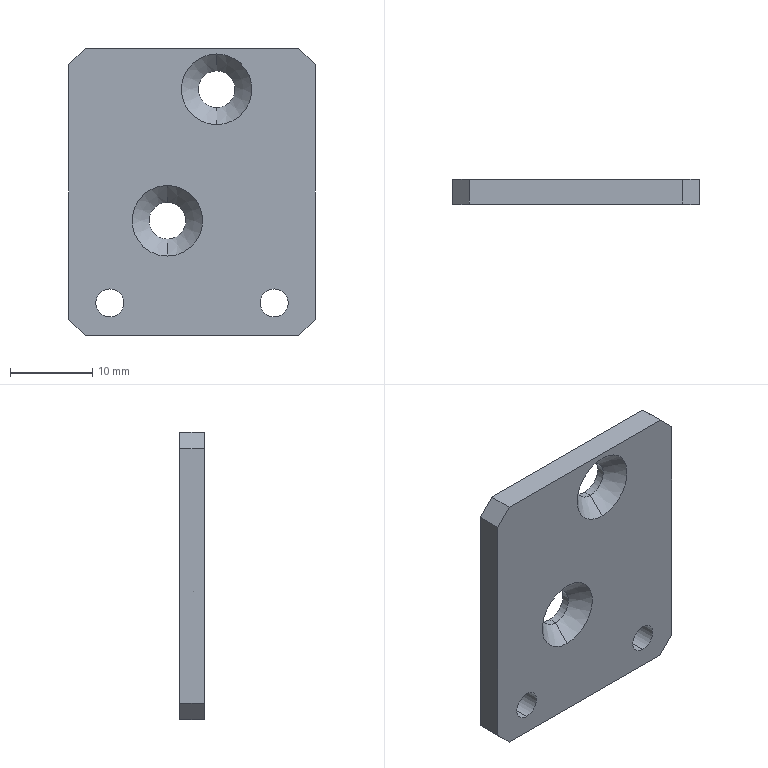Part | NX | features BREP 1 | 1 solid | 22 faces | box 30 x 3 x 35 mm | volume 2899 mm3 | plane 10 | cylinder 8 | cone 4 | commonest cylinder face diameters 3.4 x4 4.5 x4
STEP:
#1=CARTESIAN_POINT('',(-15.,-3.,-15.5));
#2=VERTEX_POINT('',#1);
#3=CARTESIAN_POINT('',(-13.,-3.,-17.5));
#4=VERTEX_POINT('',#3);
#5=CARTESIAN_POINT('',(-13.,-3.,-17.5));
#6=DIRECTION('',(0.7071,0.,-0.7071));
#7=VECTOR('',#6,1000.);
#8=LINE('',#5,#7);
#9=EDGE_CURVE('',#2,#4,#8,.T.);
#10=ORIENTED_EDGE('',*,*,#9,.F.);
#11=CARTESIAN_POINT('',(-15.,0.,-15.5));
#12=VERTEX_POINT('',#11);
#13=CARTESIAN_POINT('',(-15.,-3.,-15.5));
#14=DIRECTION('',(0.,-1.,0.));
#15=VECTOR('',#14,1000.);
#16=LINE('',#13,#15);
#17=EDGE_CURVE('',#12,#2,#16,.T.);
#18=ORIENTED_EDGE('',*,*,#17,.F.);
#19=CARTESIAN_POINT('',(-13.,0.,-17.5));
#20=VERTEX_POINT('',#19);
#21=CARTESIAN_POINT('',(-15.25,0.,-15.25));
#22=DIRECTION('',(-0.7071,0.,0.7071));
#23=VECTOR('',#22,1000.);
#24=LINE('',#21,#23);
#25=EDGE_CURVE('',#20,#12,#24,.T.);
#26=ORIENTED_EDGE('',*,*,#25,.F.);
#27=CARTESIAN_POINT('',(-13.,-3.,-17.5));
#28=DIRECTION('',(0.,1.,0.));
#29=VECTOR('',#28,1000.);
#30=LINE('',#27,#29);
#31=EDGE_CURVE('',#4,#20,#30,.T.);
#32=ORIENTED_EDGE('',*,*,#31,.F.);
#33=EDGE_LOOP('',(#10,#18,#26,#32));
#34=FACE_BOUND('',#33,.T.);
#35=CARTESIAN_POINT('',(-13.,-3.,-17.5));
#36=DIRECTION('',(0.7071,0.,0.7071));
#37=DIRECTION('',(0.,1.,0.));
#38=AXIS2_PLACEMENT_3D('',#35,#36,#37);
#39=PLANE('',#38);
#40=ADVANCED_FACE('',(#34),#39,.F.);
#41=CARTESIAN_POINT('',(13.,-3.,-17.5));
#42=VERTEX_POINT('',#41);
#43=CARTESIAN_POINT('',(15.,-3.,-15.5));
#44=VERTEX_POINT('',#43);
#45=CARTESIAN_POINT('',(15.,-3.,-15.5));
#46=DIRECTION('',(0.7071,0.,0.7071));
#47=VECTOR('',#46,1000.);
#48=LINE('',#45,#47);
#49=EDGE_CURVE('',#42,#44,#48,.T.);
#50=ORIENTED_EDGE('',*,*,#49,.F.);
#51=CARTESIAN_POINT('',(13.,0.,-17.5));
#52=VERTEX_POINT('',#51);
#53=CARTESIAN_POINT('',(13.,-3.,-17.5));
#54=DIRECTION('',(0.,-1.,0.));
#55=VECTOR('',#54,1000.);
#56=LINE('',#53,#55);
#57=EDGE_CURVE('',#52,#42,#56,.T.);
#58=ORIENTED_EDGE('',*,*,#57,.F.);
#59=CARTESIAN_POINT('',(15.,0.,-15.5));
#60=VERTEX_POINT('',#59);
#61=CARTESIAN_POINT('',(15.25,0.,-15.25));
#62=DIRECTION('',(-0.7071,0.,-0.7071));
#63=VECTOR('',#62,1000.);
#64=LINE('',#61,#63);
#65=EDGE_CURVE('',#60,#52,#64,.T.);
#66=ORIENTED_EDGE('',*,*,#65,.F.);
#67=CARTESIAN_POINT('',(15.,-3.,-15.5));
#68=DIRECTION('',(0.,1.,0.));
#69=VECTOR('',#68,1000.);
#70=LINE('',#67,#69);
#71=EDGE_CURVE('',#44,#60,#70,.T.);
#72=ORIENTED_EDGE('',*,*,#71,.F.);
#73=EDGE_LOOP('',(#50,#58,#66,#72));
#74=FACE_BOUND('',#73,.T.);
#75=CARTESIAN_POINT('',(15.,-3.,-15.5));
#76=DIRECTION('',(-0.7071,0.,0.7071));
#77=DIRECTION('',(0.,1.,0.));
#78=AXIS2_PLACEMENT_3D('',#75,#76,#77);
#79=PLANE('',#78);
#80=ADVANCED_FACE('',(#74),#79,.F.);
#81=CARTESIAN_POINT('',(15.,-3.,15.5));
#82=VERTEX_POINT('',#81);
#83=CARTESIAN_POINT('',(13.,-3.,17.5));
#84=VERTEX_POINT('',#83);
#85=CARTESIAN_POINT('',(13.,-3.,17.5));
#86=DIRECTION('',(-0.7071,0.,0.7071));
#87=VECTOR('',#86,1000.);
#88=LINE('',#85,#87);
#89=EDGE_CURVE('',#82,#84,#88,.T.);
#90=ORIENTED_EDGE('',*,*,#89,.F.);
#91=CARTESIAN_POINT('',(15.,0.,15.5));
#92=VERTEX_POINT('',#91);
#93=CARTESIAN_POINT('',(15.,-3.,15.5));
#94=DIRECTION('',(0.,-1.,0.));
#95=VECTOR('',#94,1000.);
#96=LINE('',#93,#95);
#97=EDGE_CURVE('',#92,#82,#96,.T.);
#98=ORIENTED_EDGE('',*,*,#97,.F.);
#99=CARTESIAN_POINT('',(13.,0.,17.5));
#100=VERTEX_POINT('',#99);
#101=CARTESIAN_POINT('',(15.25,0.,15.25));
#102=DIRECTION('',(0.7071,0.,-0.7071));
#103=VECTOR('',#102,1000.);
#104=LINE('',#101,#103);
#105=EDGE_CURVE('',#100,#92,#104,.T.);
#106=ORIENTED_EDGE('',*,*,#105,.F.);
#107=CARTESIAN_POINT('',(13.,-3.,17.5));
#108=DIRECTION('',(0.,1.,0.));
#109=VECTOR('',#108,1000.);
#110=LINE('',#107,#109);
#111=EDGE_CURVE('',#84,#100,#110,.T.);
#112=ORIENTED_EDGE('',*,*,#111,.F.);
#113=EDGE_LOOP('',(#90,#98,#106,#112));
#114=FACE_BOUND('',#113,.T.);
#115=CARTESIAN_POINT('',(13.,-3.,17.5));
#116=DIRECTION('',(-0.7071,0.,-0.7071));
#117=DIRECTION('',(0.,1.,0.));
#118=AXIS2_PLACEMENT_3D('',#115,#116,#117);
#119=PLANE('',#118);
#120=ADVANCED_FACE('',(#114),#119,.F.);
#121=CARTESIAN_POINT('',(-13.,-3.,17.5));
#122=VERTEX_POINT('',#121);
#123=CARTESIAN_POINT('',(-15.,-3.,15.5));
#124=VERTEX_POINT('',#123);
#125=CARTESIAN_POINT('',(-15.,-3.,15.5));
#126=DIRECTION('',(-0.7071,0.,-0.7071));
#127=VECTOR('',#126,1000.);
#128=LINE('',#125,#127);
#129=EDGE_CURVE('',#122,#124,#128,.T.);
#130=ORIENTED_EDGE('',*,*,#129,.F.);
#131=CARTESIAN_POINT('',(-13.,0.,17.5));
#132=VERTEX_POINT('',#131);
#133=CARTESIAN_POINT('',(-13.,-3.,17.5));
#134=DIRECTION('',(0.,-1.,0.));
#135=VECTOR('',#134,1000.);
#136=LINE('',#133,#135);
#137=EDGE_CURVE('',#132,#122,#136,.T.);
#138=ORIENTED_EDGE('',*,*,#137,.F.);
#139=CARTESIAN_POINT('',(-15.,0.,15.5));
#140=VERTEX_POINT('',#139);
#141=CARTESIAN_POINT('',(-15.25,0.,15.25));
#142=DIRECTION('',(0.7071,0.,0.7071));
#143=VECTOR('',#142,1000.);
#144=LINE('',#141,#143);
#145=EDGE_CURVE('',#140,#132,#144,.T.);
#146=ORIENTED_EDGE('',*,*,#145,.F.);
#147=CARTESIAN_POINT('',(-15.,-3.,15.5));
#148=DIRECTION('',(0.,1.,0.));
#149=VECTOR('',#148,1000.);
#150=LINE('',#147,#149);
#151=EDGE_CURVE('',#124,#140,#150,.T.);
#152=ORIENTED_EDGE('',*,*,#151,.F.);
#153=EDGE_LOOP('',(#130,#138,#146,#152));
#154=FACE_BOUND('',#153,.T.);
#155=CARTESIAN_POINT('',(-15.,-3.,15.5));
#156=DIRECTION('',(0.7071,0.,-0.7071));
#157=DIRECTION('',(0.,1.,0.));
#158=AXIS2_PLACEMENT_3D('',#155,#156,#157);
#159=PLANE('',#158);
#160=ADVANCED_FACE('',(#154),#159,.F.);
#161=CARTESIAN_POINT('',(-10.,0.,-15.2));
#162=VERTEX_POINT('',#161);
#163=CARTESIAN_POINT('',(-10.,-3.,-15.2));
#164=VERTEX_POINT('',#163);
#165=CARTESIAN_POINT('',(-10.,0.,-15.2));
#166=DIRECTION('',(0.,1.,0.));
#167=VECTOR('',#166,1000.);
#168=LINE('',#165,#167);
#169=EDGE_CURVE('',#162,#164,#168,.F.);
#170=ORIENTED_EDGE('',*,*,#169,.T.);
#171=CARTESIAN_POINT('',(-10.,-3.,-11.8));
#172=VERTEX_POINT('',#171);
#173=CARTESIAN_POINT('',(-10.,-3.,-13.5));
#174=DIRECTION('',(0.,1.,0.));
#175=DIRECTION('',(0.,0.,1.));
#176=AXIS2_PLACEMENT_3D('',#173,#174,#175);
#177=CIRCLE('',#176,1.7);
#178=EDGE_CURVE('',#172,#164,#177,.T.);
#179=ORIENTED_EDGE('',*,*,#178,.F.);
#180=CARTESIAN_POINT('',(-10.,0.,-11.8));
#181=VERTEX_POINT('',#180);
#182=CARTESIAN_POINT('',(-10.,0.,-11.8));
#183=DIRECTION('',(0.,1.,0.));
#184=VECTOR('',#183,1000.);
#185=LINE('',#182,#184);
#186=EDGE_CURVE('',#181,#172,#185,.F.);
#187=ORIENTED_EDGE('',*,*,#186,.F.);
#188=CARTESIAN_POINT('',(-10.,0.,-13.5));
#189=DIRECTION('',(0.,1.,0.));
#190=DIRECTION('',(0.,0.,1.));
#191=AXIS2_PLACEMENT_3D('',#188,#189,#190);
#192=CIRCLE('',#191,1.7);
#193=EDGE_CURVE('',#181,#162,#192,.T.);
#194=ORIENTED_EDGE('',*,*,#193,.T.);
#195=EDGE_LOOP('',(#170,#179,#187,#194));
#196=FACE_BOUND('',#195,.T.);
#197=CARTESIAN_POINT('',(-10.,0.,-13.5));
#198=DIRECTION('',(0.,1.,0.));
#199=DIRECTION('',(0.,0.,1.));
#200=AXIS2_PLACEMENT_3D('',#197,#198,#199);
#201=CYLINDRICAL_SURFACE('',#200,1.7);
#202=ADVANCED_FACE('',(#196),#201,.F.);
#203=CARTESIAN_POINT('',(10.,0.,-15.2));
#204=VERTEX_POINT('',#203);
#205=CARTESIAN_POINT('',(10.,-3.,-15.2));
#206=VERTEX_POINT('',#205);
#207=CARTESIAN_POINT('',(10.,0.,-15.2));
#208=DIRECTION('',(0.,1.,0.));
#209=VECTOR('',#208,1000.);
#210=LINE('',#207,#209);
#211=EDGE_CURVE('',#204,#206,#210,.F.);
#212=ORIENTED_EDGE('',*,*,#211,.T.);
#213=CARTESIAN_POINT('',(10.,-3.,-11.8));
#214=VERTEX_POINT('',#213);
#215=CARTESIAN_POINT('',(10.,-3.,-13.5));
#216=DIRECTION('',(0.,1.,0.));
#217=DIRECTION('',(0.,0.,1.));
#218=AXIS2_PLACEMENT_3D('',#215,#216,#217);
#219=CIRCLE('',#218,1.7);
#220=EDGE_CURVE('',#214,#206,#219,.T.);
#221=ORIENTED_EDGE('',*,*,#220,.F.);
#222=CARTESIAN_POINT('',(10.,0.,-11.8));
#223=VERTEX_POINT('',#222);
#224=CARTESIAN_POINT('',(10.,0.,-11.8));
#225=DIRECTION('',(0.,1.,0.));
#226=VECTOR('',#225,1000.);
#227=LINE('',#224,#226);
#228=EDGE_CURVE('',#223,#214,#227,.F.);
#229=ORIENTED_EDGE('',*,*,#228,.F.);
#230=CARTESIAN_POINT('',(10.,0.,-13.5));
#231=DIRECTION('',(0.,1.,0.));
#232=DIRECTION('',(0.,0.,1.));
#233=AXIS2_PLACEMENT_3D('',#230,#231,#232);
#234=CIRCLE('',#233,1.7);
#235=EDGE_CURVE('',#223,#204,#234,.T.);
#236=ORIENTED_EDGE('',*,*,#235,.T.);
#237=EDGE_LOOP('',(#212,#221,#229,#236));
#238=FACE_BOUND('',#237,.T.);
#239=CARTESIAN_POINT('',(10.,0.,-13.5));
#240=DIRECTION('',(0.,1.,0.));
#241=DIRECTION('',(0.,0.,1.));
#242=AXIS2_PLACEMENT_3D('',#239,#240,#241);
#243=CYLINDRICAL_SURFACE('',#242,1.7);
#244=ADVANCED_FACE('',(#238),#243,.F.);
#245=CARTESIAN_POINT('',(3.,-0.95,14.75));
#246=VERTEX_POINT('',#245);
#247=CARTESIAN_POINT('',(3.,-3.,16.8));
#248=VERTEX_POINT('',#247);
#249=CARTESIAN_POINT('',(3.,-3.,16.8));
#250=DIRECTION('',(0.,-0.7071,0.7071));
#251=VECTOR('',#250,1000.);
#252=LINE('',#249,#251);
#253=EDGE_CURVE('',#246,#248,#252,.T.);
#254=ORIENTED_EDGE('',*,*,#253,.F.);
#255=CARTESIAN_POINT('',(3.,-0.95,10.25));
#256=VERTEX_POINT('',#255);
#257=CARTESIAN_POINT('',(3.,-0.95,12.5));
#258=DIRECTION('',(0.,-1.,0.));
#259=DIRECTION('',(0.,0.,-1.));
#260=AXIS2_PLACEMENT_3D('',#257,#258,#259);
#261=CIRCLE('',#260,2.25);
#262=EDGE_CURVE('',#256,#246,#261,.T.);
#263=ORIENTED_EDGE('',*,*,#262,.F.);
#264=CARTESIAN_POINT('',(3.,-3.,8.2));
#265=VERTEX_POINT('',#264);
#266=CARTESIAN_POINT('',(3.,-3.,8.2));
#267=DIRECTION('',(0.,-0.7071,-0.7071));
#268=VECTOR('',#267,1000.);
#269=LINE('',#266,#268);
#270=EDGE_CURVE('',#256,#265,#269,.T.);
#271=ORIENTED_EDGE('',*,*,#270,.T.);
#272=CARTESIAN_POINT('',(3.,-3.,12.5));
#273=DIRECTION('',(0.,-1.,0.));
#274=DIRECTION('',(0.,0.,-1.));
#275=AXIS2_PLACEMENT_3D('',#272,#273,#274);
#276=CIRCLE('',#275,4.3);
#277=EDGE_CURVE('',#265,#248,#276,.T.);
#278=ORIENTED_EDGE('',*,*,#277,.T.);
#279=EDGE_LOOP('',(#254,#263,#271,#278));
#280=FACE_BOUND('',#279,.T.);
#281=CARTESIAN_POINT('',(3.,-3.,12.5));
#282=DIRECTION('',(0.,-1.,0.));
#283=DIRECTION('',(0.,0.,-1.));
#284=AXIS2_PLACEMENT_3D('',#281,#282,#283);
#285=CONICAL_SURFACE('',#284,4.3,0.7854);
#286=ADVANCED_FACE('',(#280),#285,.F.);
#287=CARTESIAN_POINT('',(3.,0.,14.75));
#288=VERTEX_POINT('',#287);
#289=CARTESIAN_POINT('',(3.,-3.,14.75));
#290=DIRECTION('',(0.,-1.,0.));
#291=VECTOR('',#290,1000.);
#292=LINE('',#289,#291);
#293=EDGE_CURVE('',#288,#246,#292,.T.);
#294=ORIENTED_EDGE('',*,*,#293,.F.);
#295=CARTESIAN_POINT('',(3.,0.,10.25));
#296=VERTEX_POINT('',#295);
#297=CARTESIAN_POINT('',(3.,0.,12.5));
#298=DIRECTION('',(0.,-1.,0.));
#299=DIRECTION('',(0.,0.,-1.));
#300=AXIS2_PLACEMENT_3D('',#297,#298,#299);
#301=CIRCLE('',#300,2.25);
#302=EDGE_CURVE('',#296,#288,#301,.T.);
#303=ORIENTED_EDGE('',*,*,#302,.F.);
#304=CARTESIAN_POINT('',(3.,-3.,10.25));
#305=DIRECTION('',(0.,-1.,0.));
#306=VECTOR('',#305,1000.);
#307=LINE('',#304,#306);
#308=EDGE_CURVE('',#296,#256,#307,.T.);
#309=ORIENTED_EDGE('',*,*,#308,.T.);
#310=ORIENTED_EDGE('',*,*,#262,.T.);
#311=EDGE_LOOP('',(#294,#303,#309,#310));
#312=FACE_BOUND('',#311,.T.);
#313=CARTESIAN_POINT('',(3.,-3.,12.5));
#314=DIRECTION('',(0.,-1.,0.));
#315=DIRECTION('',(0.,0.,-1.));
#316=AXIS2_PLACEMENT_3D('',#313,#314,#315);
#317=CYLINDRICAL_SURFACE('',#316,2.25);
#318=ADVANCED_FACE('',(#312),#317,.F.);
#319=CARTESIAN_POINT('',(-3.,-0.95,-1.25));
#320=VERTEX_POINT('',#319);
#321=CARTESIAN_POINT('',(-3.,-3.,0.8));
#322=VERTEX_POINT('',#321);
#323=CARTESIAN_POINT('',(-3.,-3.,0.8));
#324=DIRECTION('',(0.,-0.7071,0.7071));
#325=VECTOR('',#324,1000.);
#326=LINE('',#323,#325);
#327=EDGE_CURVE('',#320,#322,#326,.T.);
#328=ORIENTED_EDGE('',*,*,#327,.F.);
#329=CARTESIAN_POINT('',(-3.,-0.95,-5.75));
#330=VERTEX_POINT('',#329);
#331=CARTESIAN_POINT('',(-3.,-0.95,-3.5));
#332=DIRECTION('',(0.,-1.,0.));
#333=DIRECTION('',(0.,0.,-1.));
#334=AXIS2_PLACEMENT_3D('',#331,#332,#333);
#335=CIRCLE('',#334,2.25);
#336=EDGE_CURVE('',#330,#320,#335,.T.);
#337=ORIENTED_EDGE('',*,*,#336,.F.);
#338=CARTESIAN_POINT('',(-3.,-3.,-7.8));
#339=VERTEX_POINT('',#338);
#340=CARTESIAN_POINT('',(-3.,-3.,-7.8));
#341=DIRECTION('',(0.,-0.7071,-0.7071));
#342=VECTOR('',#341,1000.);
#343=LINE('',#340,#342);
#344=EDGE_CURVE('',#330,#339,#343,.T.);
#345=ORIENTED_EDGE('',*,*,#344,.T.);
#346=CARTESIAN_POINT('',(-3.,-3.,-3.5));
#347=DIRECTION('',(0.,-1.,0.));
#348=DIRECTION('',(0.,0.,-1.));
#349=AXIS2_PLACEMENT_3D('',#346,#347,#348);
#350=CIRCLE('',#349,4.3);
#351=EDGE_CURVE('',#339,#322,#350,.T.);
#352=ORIENTED_EDGE('',*,*,#351,.T.);
#353=EDGE_LOOP('',(#328,#337,#345,#352));
#354=FACE_BOUND('',#353,.T.);
#355=CARTESIAN_POINT('',(-3.,-3.,-3.5));
#356=DIRECTION('',(0.,-1.,0.));
#357=DIRECTION('',(0.,0.,-1.));
#358=AXIS2_PLACEMENT_3D('',#355,#356,#357);
#359=CONICAL_SURFACE('',#358,4.3,0.7854);
#360=ADVANCED_FACE('',(#354),#359,.F.);
#361=CARTESIAN_POINT('',(-3.,0.,-1.25));
#362=VERTEX_POINT('',#361);
#363=CARTESIAN_POINT('',(-3.,-3.,-1.25));
#364=DIRECTION('',(0.,-1.,0.));
#365=VECTOR('',#364,1000.);
#366=LINE('',#363,#365);
#367=EDGE_CURVE('',#362,#320,#366,.T.);
#368=ORIENTED_EDGE('',*,*,#367,.F.);
#369=CARTESIAN_POINT('',(-3.,0.,-5.75));
#370=VERTEX_POINT('',#369);
#371=CARTESIAN_POINT('',(-3.,0.,-3.5));
#372=DIRECTION('',(0.,-1.,0.));
#373=DIRECTION('',(0.,0.,-1.));
#374=AXIS2_PLACEMENT_3D('',#371,#372,#373);
#375=CIRCLE('',#374,2.25);
#376=EDGE_CURVE('',#370,#362,#375,.T.);
#377=ORIENTED_EDGE('',*,*,#376,.F.);
#378=CARTESIAN_POINT('',(-3.,-3.,-5.75));
#379=DIRECTION('',(0.,-1.,0.));
#380=VECTOR('',#379,1000.);
#381=LINE('',#378,#380);
#382=EDGE_CURVE('',#370,#330,#381,.T.);
#383=ORIENTED_EDGE('',*,*,#382,.T.);
#384=ORIENTED_EDGE('',*,*,#336,.T.);
#385=EDGE_LOOP('',(#368,#377,#383,#384));
#386=FACE_BOUND('',#385,.T.);
#387=CARTESIAN_POINT('',(-3.,-3.,-3.5));
#388=DIRECTION('',(0.,-1.,0.));
#389=DIRECTION('',(0.,0.,-1.));
#390=AXIS2_PLACEMENT_3D('',#387,#388,#389);
#391=CYLINDRICAL_SURFACE('',#390,2.25);
#392=ADVANCED_FACE('',(#386),#391,.F.);
#393=CARTESIAN_POINT('',(-15.,0.,-17.5));
#394=DIRECTION('',(0.,0.,1.));
#395=VECTOR('',#394,1000.);
#396=LINE('',#393,#395);
#397=EDGE_CURVE('',#12,#140,#396,.T.);
#398=ORIENTED_EDGE('',*,*,#397,.T.);
#399=ORIENTED_EDGE('',*,*,#145,.T.);
#400=CARTESIAN_POINT('',(-15.,0.,17.5));
#401=DIRECTION('',(1.,0.,0.));
#402=VECTOR('',#401,1000.);
#403=LINE('',#400,#402);
#404=EDGE_CURVE('',#132,#100,#403,.T.);
#405=ORIENTED_EDGE('',*,*,#404,.T.);
#406=ORIENTED_EDGE('',*,*,#105,.T.);
#407=CARTESIAN_POINT('',(15.,0.,-17.5));
#408=DIRECTION('',(0.,0.,-1.));
#409=VECTOR('',#408,1000.);
#410=LINE('',#407,#409);
#411=EDGE_CURVE('',#92,#60,#410,.T.);
#412=ORIENTED_EDGE('',*,*,#411,.T.);
#413=ORIENTED_EDGE('',*,*,#65,.T.);
#414=CARTESIAN_POINT('',(-15.,0.,-17.5));
#415=DIRECTION('',(-1.,0.,0.));
#416=VECTOR('',#415,1000.);
#417=LINE('',#414,#416);
#418=EDGE_CURVE('',#52,#20,#417,.T.);
#419=ORIENTED_EDGE('',*,*,#418,.T.);
#420=ORIENTED_EDGE('',*,*,#25,.T.);
#421=EDGE_LOOP('',(#398,#399,#405,#406,#412,#413,#419,#420));
#422=FACE_BOUND('',#421,.T.);
#423=ORIENTED_EDGE('',*,*,#376,.T.);
#424=CARTESIAN_POINT('',(-3.,0.,-3.5));
#425=DIRECTION('',(0.,-1.,0.));
#426=DIRECTION('',(0.,0.,-1.));
#427=AXIS2_PLACEMENT_3D('',#424,#425,#426);
#428=CIRCLE('',#427,2.25);
#429=EDGE_CURVE('',#362,#370,#428,.T.);
#430=ORIENTED_EDGE('',*,*,#429,.T.);
#431=EDGE_LOOP('',(#423,#430));
#432=FACE_BOUND('',#431,.T.);
#433=ORIENTED_EDGE('',*,*,#302,.T.);
#434=CARTESIAN_POINT('',(3.,0.,12.5));
#435=DIRECTION('',(0.,-1.,0.));
#436=DIRECTION('',(0.,0.,-1.));
#437=AXIS2_PLACEMENT_3D('',#434,#435,#436);
#438=CIRCLE('',#437,2.25);
#439=EDGE_CURVE('',#288,#296,#438,.T.);
#440=ORIENTED_EDGE('',*,*,#439,.T.);
#441=EDGE_LOOP('',(#433,#440));
#442=FACE_BOUND('',#441,.T.);
#443=ORIENTED_EDGE('',*,*,#235,.F.);
#444=CARTESIAN_POINT('',(10.,0.,-13.5));
#445=DIRECTION('',(0.,1.,0.));
#446=DIRECTION('',(0.,0.,1.));
#447=AXIS2_PLACEMENT_3D('',#444,#445,#446);
#448=CIRCLE('',#447,1.7);
#449=EDGE_CURVE('',#204,#223,#448,.T.);
#450=ORIENTED_EDGE('',*,*,#449,.F.);
#451=EDGE_LOOP('',(#443,#450));
#452=FACE_BOUND('',#451,.T.);
#453=ORIENTED_EDGE('',*,*,#193,.F.);
#454=CARTESIAN_POINT('',(-10.,0.,-13.5));
#455=DIRECTION('',(0.,1.,0.));
#456=DIRECTION('',(0.,0.,1.));
#457=AXIS2_PLACEMENT_3D('',#454,#455,#456);
#458=CIRCLE('',#457,1.7);
#459=EDGE_CURVE('',#162,#181,#458,.T.);
#460=ORIENTED_EDGE('',*,*,#459,.F.);
#461=EDGE_LOOP('',(#453,#460));
#462=FACE_BOUND('',#461,.T.);
#463=CARTESIAN_POINT('',(0.,0.,0.));
#464=DIRECTION('',(0.,1.,0.));
#465=DIRECTION('',(0.,0.,1.));
#466=AXIS2_PLACEMENT_3D('',#463,#464,#465);
#467=PLANE('',#466);
#468=ADVANCED_FACE('',(#422,#432,#442,#452,#462),#467,.T.);
#469=CARTESIAN_POINT('',(-15.,-3.,17.5));
#470=DIRECTION('',(1.,0.,0.));
#471=VECTOR('',#470,1000.);
#472=LINE('',#469,#471);
#473=EDGE_CURVE('',#122,#84,#472,.T.);
#474=ORIENTED_EDGE('',*,*,#473,.F.);
#475=ORIENTED_EDGE('',*,*,#129,.T.);
#476=CARTESIAN_POINT('',(-15.,-3.,-17.5));
#477=DIRECTION('',(0.,0.,1.));
#478=VECTOR('',#477,1000.);
#479=LINE('',#476,#478);
#480=EDGE_CURVE('',#2,#124,#479,.T.);
#481=ORIENTED_EDGE('',*,*,#480,.F.);
#482=ORIENTED_EDGE('',*,*,#9,.T.);
#483=CARTESIAN_POINT('',(-15.,-3.,-17.5));
#484=DIRECTION('',(-1.,0.,0.));
#485=VECTOR('',#484,1000.);
#486=LINE('',#483,#485);
#487=EDGE_CURVE('',#42,#4,#486,.T.);
#488=ORIENTED_EDGE('',*,*,#487,.F.);
#489=ORIENTED_EDGE('',*,*,#49,.T.);
#490=CARTESIAN_POINT('',(15.,-3.,-17.5));
#491=DIRECTION('',(0.,0.,-1.));
#492=VECTOR('',#491,1000.);
#493=LINE('',#490,#492);
#494=EDGE_CURVE('',#82,#44,#493,.T.);
#495=ORIENTED_EDGE('',*,*,#494,.F.);
#496=ORIENTED_EDGE('',*,*,#89,.T.);
#497=EDGE_LOOP('',(#474,#475,#481,#482,#488,#489,#495,#496));
#498=FACE_BOUND('',#497,.T.);
#499=ORIENTED_EDGE('',*,*,#351,.F.);
#500=CARTESIAN_POINT('',(-3.,-3.,-3.5));
#501=DIRECTION('',(0.,-1.,0.));
#502=DIRECTION('',(0.,0.,-1.));
#503=AXIS2_PLACEMENT_3D('',#500,#501,#502);
#504=CIRCLE('',#503,4.3);
#505=EDGE_CURVE('',#322,#339,#504,.T.);
#506=ORIENTED_EDGE('',*,*,#505,.F.);
#507=EDGE_LOOP('',(#499,#506));
#508=FACE_BOUND('',#507,.T.);
#509=ORIENTED_EDGE('',*,*,#277,.F.);
#510=CARTESIAN_POINT('',(3.,-3.,12.5));
#511=DIRECTION('',(0.,-1.,0.));
#512=DIRECTION('',(0.,0.,-1.));
#513=AXIS2_PLACEMENT_3D('',#510,#511,#512);
#514=CIRCLE('',#513,4.3);
#515=EDGE_CURVE('',#248,#265,#514,.T.);
#516=ORIENTED_EDGE('',*,*,#515,.F.);
#517=EDGE_LOOP('',(#509,#516));
#518=FACE_BOUND('',#517,.T.);
#519=ORIENTED_EDGE('',*,*,#220,.T.);
#520=CARTESIAN_POINT('',(10.,-3.,-13.5));
#521=DIRECTION('',(0.,1.,0.));
#522=DIRECTION('',(0.,0.,1.));
#523=AXIS2_PLACEMENT_3D('',#520,#521,#522);
#524=CIRCLE('',#523,1.7);
#525=EDGE_CURVE('',#206,#214,#524,.T.);
#526=ORIENTED_EDGE('',*,*,#525,.T.);
#527=EDGE_LOOP('',(#519,#526));
#528=FACE_BOUND('',#527,.T.);
#529=ORIENTED_EDGE('',*,*,#178,.T.);
#530=CARTESIAN_POINT('',(-10.,-3.,-13.5));
#531=DIRECTION('',(0.,1.,0.));
#532=DIRECTION('',(0.,0.,1.));
#533=AXIS2_PLACEMENT_3D('',#530,#531,#532);
#534=CIRCLE('',#533,1.7);
#535=EDGE_CURVE('',#164,#172,#534,.T.);
#536=ORIENTED_EDGE('',*,*,#535,.T.);
#537=EDGE_LOOP('',(#529,#536));
#538=FACE_BOUND('',#537,.T.);
#539=CARTESIAN_POINT('',(0.,-3.,0.));
#540=DIRECTION('',(0.,1.,0.));
#541=DIRECTION('',(0.,0.,1.));
#542=AXIS2_PLACEMENT_3D('',#539,#540,#541);
#543=PLANE('',#542);
#544=ADVANCED_FACE('',(#498,#508,#518,#528,#538),#543,.F.);
#545=ORIENTED_EDGE('',*,*,#418,.F.);
#546=ORIENTED_EDGE('',*,*,#57,.T.);
#547=ORIENTED_EDGE('',*,*,#487,.T.);
#548=ORIENTED_EDGE('',*,*,#31,.T.);
#549=EDGE_LOOP('',(#545,#546,#547,#548));
#550=FACE_BOUND('',#549,.T.);
#551=CARTESIAN_POINT('',(-15.,-3.,-17.5));
#552=DIRECTION('',(0.,0.,-1.));
#553=DIRECTION('',(-1.,0.,0.));
#554=AXIS2_PLACEMENT_3D('',#551,#552,#553);
#555=PLANE('',#554);
#556=ADVANCED_FACE('',(#550),#555,.T.);
#557=ORIENTED_EDGE('',*,*,#480,.T.);
#558=ORIENTED_EDGE('',*,*,#151,.T.);
#559=ORIENTED_EDGE('',*,*,#397,.F.);
#560=ORIENTED_EDGE('',*,*,#17,.T.);
#561=EDGE_LOOP('',(#557,#558,#559,#560));
#562=FACE_BOUND('',#561,.T.);
#563=CARTESIAN_POINT('',(-15.,-3.,-17.5));
#564=DIRECTION('',(-1.,0.,0.));
#565=DIRECTION('',(0.,0.,1.));
#566=AXIS2_PLACEMENT_3D('',#563,#564,#565);
#567=PLANE('',#566);
#568=ADVANCED_FACE('',(#562),#567,.T.);
#569=ORIENTED_EDGE('',*,*,#404,.F.);
#570=ORIENTED_EDGE('',*,*,#137,.T.);
#571=ORIENTED_EDGE('',*,*,#473,.T.);
#572=ORIENTED_EDGE('',*,*,#111,.T.);
#573=EDGE_LOOP('',(#569,#570,#571,#572));
#574=FACE_BOUND('',#573,.T.);
#575=CARTESIAN_POINT('',(-15.,-3.,17.5));
#576=DIRECTION('',(0.,0.,1.));
#577=DIRECTION('',(1.,0.,0.));
#578=AXIS2_PLACEMENT_3D('',#575,#576,#577);
#579=PLANE('',#578);
#580=ADVANCED_FACE('',(#574),#579,.T.);
#581=ORIENTED_EDGE('',*,*,#411,.F.);
#582=ORIENTED_EDGE('',*,*,#97,.T.);
#583=ORIENTED_EDGE('',*,*,#494,.T.);
#584=ORIENTED_EDGE('',*,*,#71,.T.);
#585=EDGE_LOOP('',(#581,#582,#583,#584));
#586=FACE_BOUND('',#585,.T.);
#587=CARTESIAN_POINT('',(15.,-3.,-17.5));
#588=DIRECTION('',(1.,0.,0.));
#589=DIRECTION('',(0.,0.,-1.));
#590=AXIS2_PLACEMENT_3D('',#587,#588,#589);
#591=PLANE('',#590);
#592=ADVANCED_FACE('',(#586),#591,.T.);
#593=ORIENTED_EDGE('',*,*,#429,.F.);
#594=ORIENTED_EDGE('',*,*,#367,.T.);
#595=CARTESIAN_POINT('',(-3.,-0.95,-3.5));
#596=DIRECTION('',(0.,-1.,0.));
#597=DIRECTION('',(0.,0.,-1.));
#598=AXIS2_PLACEMENT_3D('',#595,#596,#597);
#599=CIRCLE('',#598,2.25);
#600=EDGE_CURVE('',#320,#330,#599,.T.);
#601=ORIENTED_EDGE('',*,*,#600,.T.);
#602=ORIENTED_EDGE('',*,*,#382,.F.);
#603=EDGE_LOOP('',(#593,#594,#601,#602));
#604=FACE_BOUND('',#603,.T.);
#605=CARTESIAN_POINT('',(-3.,-3.,-3.5));
#606=DIRECTION('',(0.,-1.,0.));
#607=DIRECTION('',(0.,0.,-1.));
#608=AXIS2_PLACEMENT_3D('',#605,#606,#607);
#609=CYLINDRICAL_SURFACE('',#608,2.25);
#610=ADVANCED_FACE('',(#604),#609,.F.);
#611=ORIENTED_EDGE('',*,*,#600,.F.);
#612=ORIENTED_EDGE('',*,*,#327,.T.);
#613=ORIENTED_EDGE('',*,*,#505,.T.);
#614=ORIENTED_EDGE('',*,*,#344,.F.);
#615=EDGE_LOOP('',(#611,#612,#613,#614));
#616=FACE_BOUND('',#615,.T.);
#617=CARTESIAN_POINT('',(-3.,-3.,-3.5));
#618=DIRECTION('',(0.,-1.,0.));
#619=DIRECTION('',(0.,0.,-1.));
#620=AXIS2_PLACEMENT_3D('',#617,#618,#619);
#621=CONICAL_SURFACE('',#620,4.3,0.7854);
#622=ADVANCED_FACE('',(#616),#621,.F.);
#623=ORIENTED_EDGE('',*,*,#439,.F.);
#624=ORIENTED_EDGE('',*,*,#293,.T.);
#625=CARTESIAN_POINT('',(3.,-0.95,12.5));
#626=DIRECTION('',(0.,-1.,0.));
#627=DIRECTION('',(0.,0.,-1.));
#628=AXIS2_PLACEMENT_3D('',#625,#626,#627);
#629=CIRCLE('',#628,2.25);
#630=EDGE_CURVE('',#246,#256,#629,.T.);
#631=ORIENTED_EDGE('',*,*,#630,.T.);
#632=ORIENTED_EDGE('',*,*,#308,.F.);
#633=EDGE_LOOP('',(#623,#624,#631,#632));
#634=FACE_BOUND('',#633,.T.);
#635=CARTESIAN_POINT('',(3.,-3.,12.5));
#636=DIRECTION('',(0.,-1.,0.));
#637=DIRECTION('',(0.,0.,-1.));
#638=AXIS2_PLACEMENT_3D('',#635,#636,#637);
#639=CYLINDRICAL_SURFACE('',#638,2.25);
#640=ADVANCED_FACE('',(#634),#639,.F.);
#641=ORIENTED_EDGE('',*,*,#630,.F.);
#642=ORIENTED_EDGE('',*,*,#253,.T.);
#643=ORIENTED_EDGE('',*,*,#515,.T.);
#644=ORIENTED_EDGE('',*,*,#270,.F.);
#645=EDGE_LOOP('',(#641,#642,#643,#644));
#646=FACE_BOUND('',#645,.T.);
#647=CARTESIAN_POINT('',(3.,-3.,12.5));
#648=DIRECTION('',(0.,-1.,0.));
#649=DIRECTION('',(0.,0.,-1.));
#650=AXIS2_PLACEMENT_3D('',#647,#648,#649);
#651=CONICAL_SURFACE('',#650,4.3,0.7854);
#652=ADVANCED_FACE('',(#646),#651,.F.);
#653=ORIENTED_EDGE('',*,*,#525,.F.);
#654=ORIENTED_EDGE('',*,*,#211,.F.);
#655=ORIENTED_EDGE('',*,*,#449,.T.);
#656=ORIENTED_EDGE('',*,*,#228,.T.);
#657=EDGE_LOOP('',(#653,#654,#655,#656));
#658=FACE_BOUND('',#657,.T.);
#659=CARTESIAN_POINT('',(10.,0.,-13.5));
#660=DIRECTION('',(0.,1.,0.));
#661=DIRECTION('',(0.,0.,1.));
#662=AXIS2_PLACEMENT_3D('',#659,#660,#661);
#663=CYLINDRICAL_SURFACE('',#662,1.7);
#664=ADVANCED_FACE('',(#658),#663,.F.);
#665=ORIENTED_EDGE('',*,*,#535,.F.);
#666=ORIENTED_EDGE('',*,*,#169,.F.);
#667=ORIENTED_EDGE('',*,*,#459,.T.);
#668=ORIENTED_EDGE('',*,*,#186,.T.);
#669=EDGE_LOOP('',(#665,#666,#667,#668));
#670=FACE_BOUND('',#669,.T.);
#671=CARTESIAN_POINT('',(-10.,0.,-13.5));
#672=DIRECTION('',(0.,1.,0.));
#673=DIRECTION('',(0.,0.,1.));
#674=AXIS2_PLACEMENT_3D('',#671,#672,#673);
#675=CYLINDRICAL_SURFACE('',#674,1.7);
#676=ADVANCED_FACE('',(#670),#675,.F.);
#677=CLOSED_SHELL('',(#40,#80,#120,#160,#202,#244,#286,#318,#360,#392,#468,#544,#556,#568,#580,#592,#610,#622,#640,#652,#664,#676));
#678=MANIFOLD_SOLID_BREP('',#677);
#679=(LENGTH_UNIT()NAMED_UNIT(*)SI_UNIT(.MILLI.,.METRE.));
#680=UNCERTAINTY_MEASURE_WITH_UNIT(LENGTH_MEASURE(0.00001),#679,'','');
#681=(NAMED_UNIT(*)PLANE_ANGLE_UNIT()SI_UNIT($,.RADIAN.));
#682=(NAMED_UNIT(*)SI_UNIT($,.STERADIAN.)SOLID_ANGLE_UNIT());
#683=(GEOMETRIC_REPRESENTATION_CONTEXT(3)GLOBAL_UNCERTAINTY_ASSIGNED_CONTEXT((#680))GLOBAL_UNIT_ASSIGNED_CONTEXT((#679,#681,#682))REPRESENTATION_CONTEXT('',''));
#684=ADVANCED_BREP_SHAPE_REPRESENTATION('',(#678),#683);